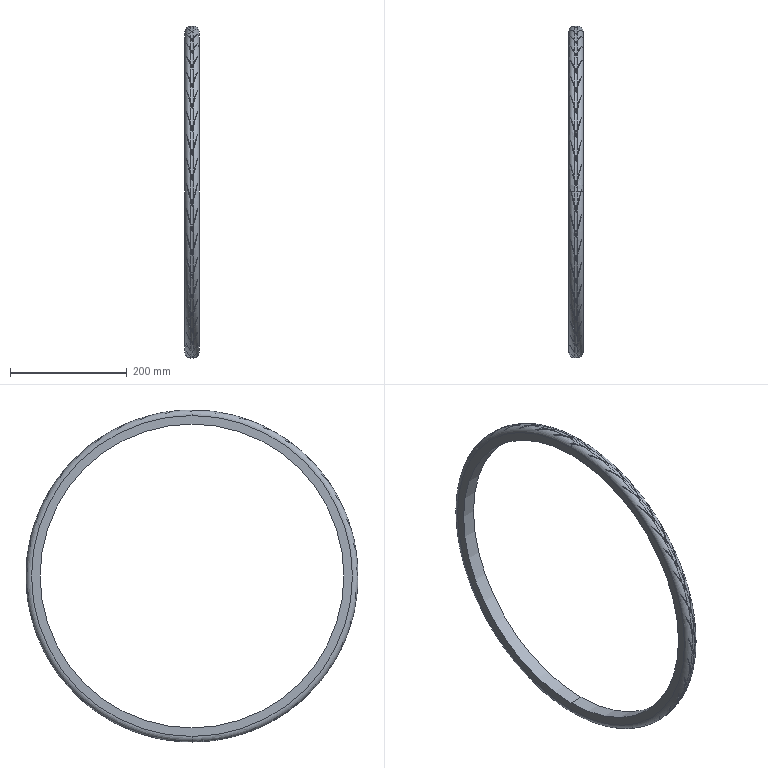Part | STEP file | Rear Royce Quick Tyre | 1 solid | 216 faces | box 24 x 568 x 568 mm | volume 911325 mm3 | spline 164 | cylinder 44 | torus 6 | plane 2 | commonest cylinder face diameters 568 x42 520 x2